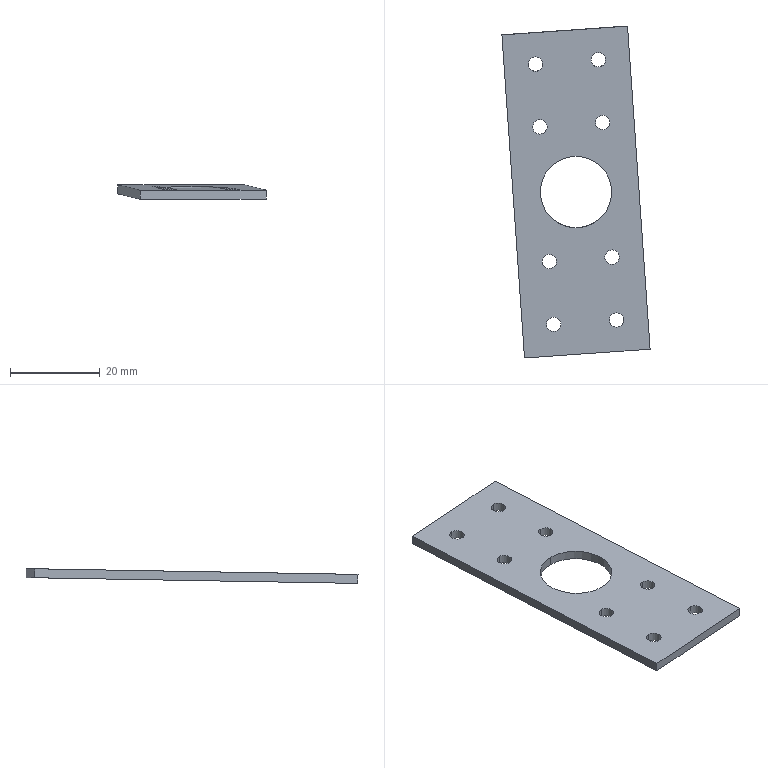Part | SolidWorks | features BaseBody 1 | 1 solid | 24 faces | box 32.959 x 73.801 x 3.287 mm | volume 3506 mm3 | cylinder 18 | plane 6 | commonest cylinder face diameters 3.2 x16 15.9 x2
STEP:
#1=CARTESIAN_POINT('',(561.633,59.844,3.845));
#2=VERTEX_POINT('',#1);
#3=CARTESIAN_POINT('',(561.633,43.947,3.568));
#4=VERTEX_POINT('',#3);
#5=CARTESIAN_POINT('',(561.633,51.896,3.706));
#6=DIRECTION('',(0.,-0.01745,0.9998));
#7=DIRECTION('',(0.,0.9998,0.01745));
#8=AXIS2_PLACEMENT_3D('',#5,#6,#7);
#9=CIRCLE('',#8,7.95);
#10=EDGE_CURVE('',#2,#4,#9,.T.);
#11=ORIENTED_EDGE('',*,*,#10,.T.);
#12=CARTESIAN_POINT('',(561.633,43.982,1.568));
#13=VERTEX_POINT('',#12);
#14=CARTESIAN_POINT('',(561.633,43.947,3.568));
#15=DIRECTION('',(0.,0.01745,-0.9998));
#16=VECTOR('',#15,1000.);
#17=LINE('',#14,#16);
#18=EDGE_CURVE('',#4,#13,#17,.T.);
#19=ORIENTED_EDGE('',*,*,#18,.T.);
#20=CARTESIAN_POINT('',(561.633,59.879,1.845));
#21=VERTEX_POINT('',#20);
#22=CARTESIAN_POINT('',(561.633,51.931,1.707));
#23=DIRECTION('',(0.,0.01745,-0.9998));
#24=DIRECTION('',(0.,0.9998,0.01745));
#25=AXIS2_PLACEMENT_3D('',#22,#23,#24);
#26=CIRCLE('',#25,7.95);
#27=EDGE_CURVE('',#13,#21,#26,.T.);
#28=ORIENTED_EDGE('',*,*,#27,.T.);
#29=CARTESIAN_POINT('',(561.633,59.844,3.845));
#30=DIRECTION('',(0.,0.01745,-0.9998));
#31=VECTOR('',#30,1000.);
#32=LINE('',#29,#31);
#33=EDGE_CURVE('',#2,#21,#32,.T.);
#34=ORIENTED_EDGE('',*,*,#33,.F.);
#35=EDGE_LOOP('',(#11,#19,#28,#34));
#36=FACE_OUTER_BOUND('',#35,.T.);
#37=CARTESIAN_POINT('',(561.633,51.896,3.706));
#38=DIRECTION('',(0.,0.01745,-0.9998));
#39=DIRECTION('',(0.,0.9998,0.01745));
#40=AXIS2_PLACEMENT_3D('',#37,#38,#39);
#41=CYLINDRICAL_SURFACE('',#40,7.95);
#42=ADVANCED_FACE('',(#36),#41,.F.);
#43=CARTESIAN_POINT('',(556.675,24.084,3.221));
#44=VERTEX_POINT('',#43);
#45=CARTESIAN_POINT('',(556.675,20.885,3.165));
#46=VERTEX_POINT('',#45);
#47=CARTESIAN_POINT('',(556.675,22.484,3.193));
#48=DIRECTION('',(0.,-0.01745,0.9998));
#49=DIRECTION('',(0.,0.9998,0.01745));
#50=AXIS2_PLACEMENT_3D('',#47,#48,#49);
#51=CIRCLE('',#50,1.6);
#52=EDGE_CURVE('',#44,#46,#51,.T.);
#53=ORIENTED_EDGE('',*,*,#52,.T.);
#54=CARTESIAN_POINT('',(556.675,20.92,1.165));
#55=VERTEX_POINT('',#54);
#56=CARTESIAN_POINT('',(556.675,20.885,3.165));
#57=DIRECTION('',(0.,0.01745,-0.9998));
#58=VECTOR('',#57,1000.);
#59=LINE('',#56,#58);
#60=EDGE_CURVE('',#46,#55,#59,.T.);
#61=ORIENTED_EDGE('',*,*,#60,.T.);
#62=CARTESIAN_POINT('',(556.675,24.119,1.221));
#63=VERTEX_POINT('',#62);
#64=CARTESIAN_POINT('',(556.675,22.519,1.193));
#65=DIRECTION('',(0.,-0.01745,0.9998));
#66=DIRECTION('',(0.,0.9998,0.01745));
#67=AXIS2_PLACEMENT_3D('',#64,#65,#66);
#68=CIRCLE('',#67,1.6);
#69=EDGE_CURVE('',#63,#55,#68,.T.);
#70=ORIENTED_EDGE('',*,*,#69,.F.);
#71=CARTESIAN_POINT('',(556.675,24.084,3.221));
#72=DIRECTION('',(0.,0.01745,-0.9998));
#73=VECTOR('',#72,1000.);
#74=LINE('',#71,#73);
#75=EDGE_CURVE('',#44,#63,#74,.T.);
#76=ORIENTED_EDGE('',*,*,#75,.F.);
#77=EDGE_LOOP('',(#53,#61,#70,#76));
#78=FACE_OUTER_BOUND('',#77,.T.);
#79=CARTESIAN_POINT('',(556.675,22.484,3.193));
#80=DIRECTION('',(0.,0.01745,-0.9998));
#81=DIRECTION('',(0.,0.9998,0.01745));
#82=AXIS2_PLACEMENT_3D('',#79,#80,#81);
#83=CYLINDRICAL_SURFACE('',#82,1.6);
#84=ADVANCED_FACE('',(#78),#83,.F.);
#85=CARTESIAN_POINT('',(555.698,38.048,3.465));
#86=VERTEX_POINT('',#85);
#87=CARTESIAN_POINT('',(555.698,34.848,3.409));
#88=VERTEX_POINT('',#87);
#89=CARTESIAN_POINT('',(555.698,36.448,3.437));
#90=DIRECTION('',(0.,-0.01745,0.9998));
#91=DIRECTION('',(0.,0.9998,0.01745));
#92=AXIS2_PLACEMENT_3D('',#89,#90,#91);
#93=CIRCLE('',#92,1.6);
#94=EDGE_CURVE('',#86,#88,#93,.T.);
#95=ORIENTED_EDGE('',*,*,#94,.T.);
#96=CARTESIAN_POINT('',(555.698,34.883,1.409));
#97=VERTEX_POINT('',#96);
#98=CARTESIAN_POINT('',(555.698,34.848,3.409));
#99=DIRECTION('',(0.,0.01745,-0.9998));
#100=VECTOR('',#99,1000.);
#101=LINE('',#98,#100);
#102=EDGE_CURVE('',#88,#97,#101,.T.);
#103=ORIENTED_EDGE('',*,*,#102,.T.);
#104=CARTESIAN_POINT('',(555.698,38.083,1.465));
#105=VERTEX_POINT('',#104);
#106=CARTESIAN_POINT('',(555.698,36.483,1.437));
#107=DIRECTION('',(0.,-0.01745,0.9998));
#108=DIRECTION('',(0.,0.9998,0.01745));
#109=AXIS2_PLACEMENT_3D('',#106,#107,#108);
#110=CIRCLE('',#109,1.6);
#111=EDGE_CURVE('',#105,#97,#110,.T.);
#112=ORIENTED_EDGE('',*,*,#111,.F.);
#113=CARTESIAN_POINT('',(555.698,38.048,3.465));
#114=DIRECTION('',(0.,0.01745,-0.9998));
#115=VECTOR('',#114,1000.);
#116=LINE('',#113,#115);
#117=EDGE_CURVE('',#86,#105,#116,.T.);
#118=ORIENTED_EDGE('',*,*,#117,.F.);
#119=EDGE_LOOP('',(#95,#103,#112,#118));
#120=FACE_OUTER_BOUND('',#119,.T.);
#121=CARTESIAN_POINT('',(555.698,36.448,3.437));
#122=DIRECTION('',(0.,0.01745,-0.9998));
#123=DIRECTION('',(0.,0.9998,0.01745));
#124=AXIS2_PLACEMENT_3D('',#121,#122,#123);
#125=CYLINDRICAL_SURFACE('',#124,1.6);
#126=ADVANCED_FACE('',(#120),#125,.F.);
#127=CARTESIAN_POINT('',(567.572,68.942,4.004));
#128=VERTEX_POINT('',#127);
#129=CARTESIAN_POINT('',(567.572,65.742,3.948));
#130=VERTEX_POINT('',#129);
#131=CARTESIAN_POINT('',(567.572,67.342,3.976));
#132=DIRECTION('',(0.,-0.01745,0.9998));
#133=DIRECTION('',(0.,0.9998,0.01745));
#134=AXIS2_PLACEMENT_3D('',#131,#132,#133);
#135=CIRCLE('',#134,1.6);
#136=EDGE_CURVE('',#128,#130,#135,.T.);
#137=ORIENTED_EDGE('',*,*,#136,.T.);
#138=CARTESIAN_POINT('',(567.572,65.777,1.948));
#139=VERTEX_POINT('',#138);
#140=CARTESIAN_POINT('',(567.572,65.742,3.948));
#141=DIRECTION('',(0.,0.01745,-0.9998));
#142=VECTOR('',#141,1000.);
#143=LINE('',#140,#142);
#144=EDGE_CURVE('',#130,#139,#143,.T.);
#145=ORIENTED_EDGE('',*,*,#144,.T.);
#146=CARTESIAN_POINT('',(567.572,68.977,2.004));
#147=VERTEX_POINT('',#146);
#148=CARTESIAN_POINT('',(567.572,67.377,1.976));
#149=DIRECTION('',(0.,-0.01745,0.9998));
#150=DIRECTION('',(0.,0.9998,0.01745));
#151=AXIS2_PLACEMENT_3D('',#148,#149,#150);
#152=CIRCLE('',#151,1.6);
#153=EDGE_CURVE('',#147,#139,#152,.T.);
#154=ORIENTED_EDGE('',*,*,#153,.F.);
#155=CARTESIAN_POINT('',(567.572,68.942,4.004));
#156=DIRECTION('',(0.,0.01745,-0.9998));
#157=VECTOR('',#156,1000.);
#158=LINE('',#155,#157);
#159=EDGE_CURVE('',#128,#147,#158,.T.);
#160=ORIENTED_EDGE('',*,*,#159,.F.);
#161=EDGE_LOOP('',(#137,#145,#154,#160));
#162=FACE_OUTER_BOUND('',#161,.T.);
#163=CARTESIAN_POINT('',(567.572,67.342,3.976));
#164=DIRECTION('',(0.,0.01745,-0.9998));
#165=DIRECTION('',(0.,0.9998,0.01745));
#166=AXIS2_PLACEMENT_3D('',#163,#164,#165);
#167=CYLINDRICAL_SURFACE('',#166,1.6);
#168=ADVANCED_FACE('',(#162),#167,.F.);
#169=CARTESIAN_POINT('',(566.596,82.906,4.248));
#170=VERTEX_POINT('',#169);
#171=CARTESIAN_POINT('',(566.596,79.706,4.192));
#172=VERTEX_POINT('',#171);
#173=CARTESIAN_POINT('',(566.596,81.306,4.22));
#174=DIRECTION('',(0.,-0.01745,0.9998));
#175=DIRECTION('',(0.,0.9998,0.01745));
#176=AXIS2_PLACEMENT_3D('',#173,#174,#175);
#177=CIRCLE('',#176,1.6);
#178=EDGE_CURVE('',#170,#172,#177,.T.);
#179=ORIENTED_EDGE('',*,*,#178,.T.);
#180=CARTESIAN_POINT('',(566.596,79.741,2.192));
#181=VERTEX_POINT('',#180);
#182=CARTESIAN_POINT('',(566.596,79.706,4.192));
#183=DIRECTION('',(0.,0.01745,-0.9998));
#184=VECTOR('',#183,1000.);
#185=LINE('',#182,#184);
#186=EDGE_CURVE('',#172,#181,#185,.T.);
#187=ORIENTED_EDGE('',*,*,#186,.T.);
#188=CARTESIAN_POINT('',(566.596,82.941,2.248));
#189=VERTEX_POINT('',#188);
#190=CARTESIAN_POINT('',(566.596,81.341,2.22));
#191=DIRECTION('',(0.,-0.01745,0.9998));
#192=DIRECTION('',(0.,0.9998,0.01745));
#193=AXIS2_PLACEMENT_3D('',#190,#191,#192);
#194=CIRCLE('',#193,1.6);
#195=EDGE_CURVE('',#189,#181,#194,.T.);
#196=ORIENTED_EDGE('',*,*,#195,.F.);
#197=CARTESIAN_POINT('',(566.596,82.906,4.248));
#198=DIRECTION('',(0.,0.01745,-0.9998));
#199=VECTOR('',#198,1000.);
#200=LINE('',#197,#199);
#201=EDGE_CURVE('',#170,#189,#200,.T.);
#202=ORIENTED_EDGE('',*,*,#201,.F.);
#203=EDGE_LOOP('',(#179,#187,#196,#202));
#204=FACE_OUTER_BOUND('',#203,.T.);
#205=CARTESIAN_POINT('',(566.596,81.306,4.22));
#206=DIRECTION('',(0.,0.01745,-0.9998));
#207=DIRECTION('',(0.,0.9998,0.01745));
#208=AXIS2_PLACEMENT_3D('',#205,#206,#207);
#209=CYLINDRICAL_SURFACE('',#208,1.6);
#210=ADVANCED_FACE('',(#204),#209,.F.);
#211=CARTESIAN_POINT('',(552.63,81.931,4.231));
#212=VERTEX_POINT('',#211);
#213=CARTESIAN_POINT('',(552.63,78.731,4.175));
#214=VERTEX_POINT('',#213);
#215=CARTESIAN_POINT('',(552.63,80.331,4.203));
#216=DIRECTION('',(0.,-0.01745,0.9998));
#217=DIRECTION('',(0.,0.9998,0.01745));
#218=AXIS2_PLACEMENT_3D('',#215,#216,#217);
#219=CIRCLE('',#218,1.6);
#220=EDGE_CURVE('',#212,#214,#219,.T.);
#221=ORIENTED_EDGE('',*,*,#220,.T.);
#222=CARTESIAN_POINT('',(552.63,78.766,2.175));
#223=VERTEX_POINT('',#222);
#224=CARTESIAN_POINT('',(552.63,78.731,4.175));
#225=DIRECTION('',(0.,0.01745,-0.9998));
#226=VECTOR('',#225,1000.);
#227=LINE('',#224,#226);
#228=EDGE_CURVE('',#214,#223,#227,.T.);
#229=ORIENTED_EDGE('',*,*,#228,.T.);
#230=CARTESIAN_POINT('',(552.63,81.966,2.231));
#231=VERTEX_POINT('',#230);
#232=CARTESIAN_POINT('',(552.63,80.366,2.203));
#233=DIRECTION('',(0.,-0.01745,0.9998));
#234=DIRECTION('',(0.,0.9998,0.01745));
#235=AXIS2_PLACEMENT_3D('',#232,#233,#234);
#236=CIRCLE('',#235,1.6);
#237=EDGE_CURVE('',#231,#223,#236,.T.);
#238=ORIENTED_EDGE('',*,*,#237,.F.);
#239=CARTESIAN_POINT('',(552.63,81.931,4.231));
#240=DIRECTION('',(0.,0.01745,-0.9998));
#241=VECTOR('',#240,1000.);
#242=LINE('',#239,#241);
#243=EDGE_CURVE('',#212,#231,#242,.T.);
#244=ORIENTED_EDGE('',*,*,#243,.F.);
#245=EDGE_LOOP('',(#221,#229,#238,#244));
#246=FACE_OUTER_BOUND('',#245,.T.);
#247=CARTESIAN_POINT('',(552.63,80.331,4.203));
#248=DIRECTION('',(0.,0.01745,-0.9998));
#249=DIRECTION('',(0.,0.9998,0.01745));
#250=AXIS2_PLACEMENT_3D('',#247,#248,#249);
#251=CYLINDRICAL_SURFACE('',#250,1.6);
#252=ADVANCED_FACE('',(#246),#251,.F.);
#253=CARTESIAN_POINT('',(553.606,67.967,3.987));
#254=VERTEX_POINT('',#253);
#255=CARTESIAN_POINT('',(553.606,64.767,3.931));
#256=VERTEX_POINT('',#255);
#257=CARTESIAN_POINT('',(553.606,66.367,3.959));
#258=DIRECTION('',(0.,-0.01745,0.9998));
#259=DIRECTION('',(0.,0.9998,0.01745));
#260=AXIS2_PLACEMENT_3D('',#257,#258,#259);
#261=CIRCLE('',#260,1.6);
#262=EDGE_CURVE('',#254,#256,#261,.T.);
#263=ORIENTED_EDGE('',*,*,#262,.T.);
#264=CARTESIAN_POINT('',(553.606,64.802,1.931));
#265=VERTEX_POINT('',#264);
#266=CARTESIAN_POINT('',(553.606,64.767,3.931));
#267=DIRECTION('',(0.,0.01745,-0.9998));
#268=VECTOR('',#267,1000.);
#269=LINE('',#266,#268);
#270=EDGE_CURVE('',#256,#265,#269,.T.);
#271=ORIENTED_EDGE('',*,*,#270,.T.);
#272=CARTESIAN_POINT('',(553.606,68.002,1.987));
#273=VERTEX_POINT('',#272);
#274=CARTESIAN_POINT('',(553.606,66.402,1.959));
#275=DIRECTION('',(0.,-0.01745,0.9998));
#276=DIRECTION('',(0.,0.9998,0.01745));
#277=AXIS2_PLACEMENT_3D('',#274,#275,#276);
#278=CIRCLE('',#277,1.6);
#279=EDGE_CURVE('',#273,#265,#278,.T.);
#280=ORIENTED_EDGE('',*,*,#279,.F.);
#281=CARTESIAN_POINT('',(553.606,67.967,3.987));
#282=DIRECTION('',(0.,0.01745,-0.9998));
#283=VECTOR('',#282,1000.);
#284=LINE('',#281,#283);
#285=EDGE_CURVE('',#254,#273,#284,.T.);
#286=ORIENTED_EDGE('',*,*,#285,.F.);
#287=EDGE_LOOP('',(#263,#271,#280,#286));
#288=FACE_OUTER_BOUND('',#287,.T.);
#289=CARTESIAN_POINT('',(553.606,66.367,3.959));
#290=DIRECTION('',(0.,0.01745,-0.9998));
#291=DIRECTION('',(0.,0.9998,0.01745));
#292=AXIS2_PLACEMENT_3D('',#289,#290,#291);
#293=CYLINDRICAL_SURFACE('',#292,1.6);
#294=ADVANCED_FACE('',(#288),#293,.F.);
#295=CARTESIAN_POINT('',(569.663,39.025,3.482));
#296=VERTEX_POINT('',#295);
#297=CARTESIAN_POINT('',(569.663,35.826,3.426));
#298=VERTEX_POINT('',#297);
#299=CARTESIAN_POINT('',(569.663,37.425,3.454));
#300=DIRECTION('',(0.,-0.01745,0.9998));
#301=DIRECTION('',(0.,0.9998,0.01745));
#302=AXIS2_PLACEMENT_3D('',#299,#300,#301);
#303=CIRCLE('',#302,1.6);
#304=EDGE_CURVE('',#296,#298,#303,.T.);
#305=ORIENTED_EDGE('',*,*,#304,.T.);
#306=CARTESIAN_POINT('',(569.663,35.861,1.426));
#307=VERTEX_POINT('',#306);
#308=CARTESIAN_POINT('',(569.663,35.826,3.426));
#309=DIRECTION('',(0.,0.01745,-0.9998));
#310=VECTOR('',#309,1000.);
#311=LINE('',#308,#310);
#312=EDGE_CURVE('',#298,#307,#311,.T.);
#313=ORIENTED_EDGE('',*,*,#312,.T.);
#314=CARTESIAN_POINT('',(569.663,39.06,1.482));
#315=VERTEX_POINT('',#314);
#316=CARTESIAN_POINT('',(569.663,37.46,1.454));
#317=DIRECTION('',(0.,-0.01745,0.9998));
#318=DIRECTION('',(0.,0.9998,0.01745));
#319=AXIS2_PLACEMENT_3D('',#316,#317,#318);
#320=CIRCLE('',#319,1.6);
#321=EDGE_CURVE('',#315,#307,#320,.T.);
#322=ORIENTED_EDGE('',*,*,#321,.F.);
#323=CARTESIAN_POINT('',(569.663,39.025,3.482));
#324=DIRECTION('',(0.,0.01745,-0.9998));
#325=VECTOR('',#324,1000.);
#326=LINE('',#323,#325);
#327=EDGE_CURVE('',#296,#315,#326,.T.);
#328=ORIENTED_EDGE('',*,*,#327,.F.);
#329=EDGE_LOOP('',(#305,#313,#322,#328));
#330=FACE_OUTER_BOUND('',#329,.T.);
#331=CARTESIAN_POINT('',(569.663,37.425,3.454));
#332=DIRECTION('',(0.,0.01745,-0.9998));
#333=DIRECTION('',(0.,0.9998,0.01745));
#334=AXIS2_PLACEMENT_3D('',#331,#332,#333);
#335=CYLINDRICAL_SURFACE('',#334,1.6);
#336=ADVANCED_FACE('',(#330),#335,.F.);
#337=CARTESIAN_POINT('',(570.641,25.062,3.238));
#338=VERTEX_POINT('',#337);
#339=CARTESIAN_POINT('',(570.641,21.862,3.182));
#340=VERTEX_POINT('',#339);
#341=CARTESIAN_POINT('',(570.641,23.462,3.21));
#342=DIRECTION('',(0.,-0.01745,0.9998));
#343=DIRECTION('',(0.,0.9998,0.01745));
#344=AXIS2_PLACEMENT_3D('',#341,#342,#343);
#345=CIRCLE('',#344,1.6);
#346=EDGE_CURVE('',#338,#340,#345,.T.);
#347=ORIENTED_EDGE('',*,*,#346,.T.);
#348=CARTESIAN_POINT('',(570.641,21.897,1.182));
#349=VERTEX_POINT('',#348);
#350=CARTESIAN_POINT('',(570.641,21.862,3.182));
#351=DIRECTION('',(0.,0.01745,-0.9998));
#352=VECTOR('',#351,1000.);
#353=LINE('',#350,#352);
#354=EDGE_CURVE('',#340,#349,#353,.T.);
#355=ORIENTED_EDGE('',*,*,#354,.T.);
#356=CARTESIAN_POINT('',(570.641,25.096,1.238));
#357=VERTEX_POINT('',#356);
#358=CARTESIAN_POINT('',(570.641,23.497,1.21));
#359=DIRECTION('',(0.,-0.01745,0.9998));
#360=DIRECTION('',(0.,0.9998,0.01745));
#361=AXIS2_PLACEMENT_3D('',#358,#359,#360);
#362=CIRCLE('',#361,1.6);
#363=EDGE_CURVE('',#357,#349,#362,.T.);
#364=ORIENTED_EDGE('',*,*,#363,.F.);
#365=CARTESIAN_POINT('',(570.641,25.062,3.238));
#366=DIRECTION('',(0.,0.01745,-0.9998));
#367=VECTOR('',#366,1000.);
#368=LINE('',#365,#367);
#369=EDGE_CURVE('',#338,#357,#368,.T.);
#370=ORIENTED_EDGE('',*,*,#369,.F.);
#371=EDGE_LOOP('',(#347,#355,#364,#370));
#372=FACE_OUTER_BOUND('',#371,.T.);
#373=CARTESIAN_POINT('',(570.641,23.462,3.21));
#374=DIRECTION('',(0.,0.01745,-0.9998));
#375=DIRECTION('',(0.,0.9998,0.01745));
#376=AXIS2_PLACEMENT_3D('',#373,#374,#375);
#377=CYLINDRICAL_SURFACE('',#376,1.6);
#378=ADVANCED_FACE('',(#372),#377,.F.);
#379=ORIENTED_EDGE('',*,*,#18,.F.);
#380=CARTESIAN_POINT('',(561.633,51.896,3.706));
#381=DIRECTION('',(0.,-0.01745,0.9998));
#382=DIRECTION('',(0.,0.9998,0.01745));
#383=AXIS2_PLACEMENT_3D('',#380,#381,#382);
#384=CIRCLE('',#383,7.95);
#385=EDGE_CURVE('',#4,#2,#384,.T.);
#386=ORIENTED_EDGE('',*,*,#385,.T.);
#387=ORIENTED_EDGE('',*,*,#33,.T.);
#388=CARTESIAN_POINT('',(561.633,51.931,1.707));
#389=DIRECTION('',(0.,0.01745,-0.9998));
#390=DIRECTION('',(0.,0.9998,0.01745));
#391=AXIS2_PLACEMENT_3D('',#388,#389,#390);
#392=CIRCLE('',#391,7.95);
#393=EDGE_CURVE('',#21,#13,#392,.T.);
#394=ORIENTED_EDGE('',*,*,#393,.T.);
#395=EDGE_LOOP('',(#379,#386,#387,#394));
#396=FACE_OUTER_BOUND('',#395,.T.);
#397=CARTESIAN_POINT('',(561.633,51.896,3.706));
#398=DIRECTION('',(0.,0.01745,-0.9998));
#399=DIRECTION('',(0.,0.9998,0.01745));
#400=AXIS2_PLACEMENT_3D('',#397,#398,#399);
#401=CYLINDRICAL_SURFACE('',#400,7.95);
#402=ADVANCED_FACE('',(#396),#401,.F.);
#403=ORIENTED_EDGE('',*,*,#393,.F.);
#404=ORIENTED_EDGE('',*,*,#27,.F.);
#405=EDGE_LOOP('',(#403,#404));
#406=FACE_BOUND('',#405,.T.);
#407=ORIENTED_EDGE('',*,*,#69,.T.);
#408=CARTESIAN_POINT('',(556.675,22.519,1.193));
#409=DIRECTION('',(0.,-0.01745,0.9998));
#410=DIRECTION('',(0.,0.9998,0.01745));
#411=AXIS2_PLACEMENT_3D('',#408,#409,#410);
#412=CIRCLE('',#411,1.6);
#413=EDGE_CURVE('',#55,#63,#412,.T.);
#414=ORIENTED_EDGE('',*,*,#413,.T.);
#415=EDGE_LOOP('',(#407,#414));
#416=FACE_BOUND('',#415,.T.);
#417=ORIENTED_EDGE('',*,*,#111,.T.);
#418=CARTESIAN_POINT('',(555.698,36.483,1.437));
#419=DIRECTION('',(0.,-0.01745,0.9998));
#420=DIRECTION('',(0.,0.9998,0.01745));
#421=AXIS2_PLACEMENT_3D('',#418,#419,#420);
#422=CIRCLE('',#421,1.6);
#423=EDGE_CURVE('',#97,#105,#422,.T.);
#424=ORIENTED_EDGE('',*,*,#423,.T.);
#425=EDGE_LOOP('',(#417,#424));
#426=FACE_BOUND('',#425,.T.);
#427=ORIENTED_EDGE('',*,*,#153,.T.);
#428=CARTESIAN_POINT('',(567.572,67.377,1.976));
#429=DIRECTION('',(0.,-0.01745,0.9998));
#430=DIRECTION('',(0.,0.9998,0.01745));
#431=AXIS2_PLACEMENT_3D('',#428,#429,#430);
#432=CIRCLE('',#431,1.6);
#433=EDGE_CURVE('',#139,#147,#432,.T.);
#434=ORIENTED_EDGE('',*,*,#433,.T.);
#435=EDGE_LOOP('',(#427,#434));
#436=FACE_BOUND('',#435,.T.);
#437=ORIENTED_EDGE('',*,*,#195,.T.);
#438=CARTESIAN_POINT('',(566.596,81.341,2.22));
#439=DIRECTION('',(0.,-0.01745,0.9998));
#440=DIRECTION('',(0.,0.9998,0.01745));
#441=AXIS2_PLACEMENT_3D('',#438,#439,#440);
#442=CIRCLE('',#441,1.6);
#443=EDGE_CURVE('',#181,#189,#442,.T.);
#444=ORIENTED_EDGE('',*,*,#443,.T.);
#445=EDGE_LOOP('',(#437,#444));
#446=FACE_BOUND('',#445,.T.);
#447=ORIENTED_EDGE('',*,*,#237,.T.);
#448=CARTESIAN_POINT('',(552.63,80.366,2.203));
#449=DIRECTION('',(0.,-0.01745,0.9998));
#450=DIRECTION('',(0.,0.9998,0.01745));
#451=AXIS2_PLACEMENT_3D('',#448,#449,#450);
#452=CIRCLE('',#451,1.6);
#453=EDGE_CURVE('',#223,#231,#452,.T.);
#454=ORIENTED_EDGE('',*,*,#453,.T.);
#455=EDGE_LOOP('',(#447,#454));
#456=FACE_BOUND('',#455,.T.);
#457=ORIENTED_EDGE('',*,*,#279,.T.);
#458=CARTESIAN_POINT('',(553.606,66.402,1.959));
#459=DIRECTION('',(0.,-0.01745,0.9998));
#460=DIRECTION('',(0.,0.9998,0.01745));
#461=AXIS2_PLACEMENT_3D('',#458,#459,#460);
#462=CIRCLE('',#461,1.6);
#463=EDGE_CURVE('',#265,#273,#462,.T.);
#464=ORIENTED_EDGE('',*,*,#463,.T.);
#465=EDGE_LOOP('',(#457,#464));
#466=FACE_BOUND('',#465,.T.);
#467=ORIENTED_EDGE('',*,*,#321,.T.);
#468=CARTESIAN_POINT('',(569.663,37.46,1.454));
#469=DIRECTION('',(0.,-0.01745,0.9998));
#470=DIRECTION('',(0.,0.9998,0.01745));
#471=AXIS2_PLACEMENT_3D('',#468,#469,#470);
#472=CIRCLE('',#471,1.6);
#473=EDGE_CURVE('',#307,#315,#472,.T.);
#474=ORIENTED_EDGE('',*,*,#473,.T.);
#475=EDGE_LOOP('',(#467,#474));
#476=FACE_BOUND('',#475,.T.);
#477=ORIENTED_EDGE('',*,*,#363,.T.);
#478=CARTESIAN_POINT('',(570.641,23.497,1.21));
#479=DIRECTION('',(0.,-0.01745,0.9998));
#480=DIRECTION('',(0.,0.9998,0.01745));
#481=AXIS2_PLACEMENT_3D('',#478,#479,#480);
#482=CIRCLE('',#481,1.6);
#483=EDGE_CURVE('',#349,#357,#482,.T.);
#484=ORIENTED_EDGE('',*,*,#483,.T.);
#485=EDGE_LOOP('',(#477,#484));
#486=FACE_BOUND('',#485,.T.);
#487=CARTESIAN_POINT('',(550.181,15.049,1.063));
#488=VERTEX_POINT('',#487);
#489=CARTESIAN_POINT('',(545.154,86.86,2.316));
#490=VERTEX_POINT('',#489);
#491=CARTESIAN_POINT('',(550.181,15.049,1.063));
#492=DIRECTION('',(-0.06982,0.9974,0.01741));
#493=VECTOR('',#492,1000.);
#494=LINE('',#491,#493);
#495=EDGE_CURVE('',#488,#490,#494,.T.);
#496=ORIENTED_EDGE('',*,*,#495,.T.);
#497=CARTESIAN_POINT('',(573.086,88.815,2.35));
#498=VERTEX_POINT('',#497);
#499=CARTESIAN_POINT('',(545.154,86.86,2.316));
#500=DIRECTION('',(0.9976,0.06981,0.001219));
#501=VECTOR('',#500,1000.);
#502=LINE('',#499,#501);
#503=EDGE_CURVE('',#490,#498,#502,.T.);
#504=ORIENTED_EDGE('',*,*,#503,.T.);
#505=CARTESIAN_POINT('',(578.113,17.003,1.097));
#506=VERTEX_POINT('',#505);
#507=CARTESIAN_POINT('',(573.086,88.815,2.35));
#508=DIRECTION('',(0.06982,-0.9974,-0.01741));
#509=VECTOR('',#508,1000.);
#510=LINE('',#507,#509);
#511=EDGE_CURVE('',#498,#506,#510,.T.);
#512=ORIENTED_EDGE('',*,*,#511,.T.);
#513=CARTESIAN_POINT('',(578.113,17.003,1.097));
#514=DIRECTION('',(-0.9976,-0.06981,-0.001219));
#515=VECTOR('',#514,1000.);
#516=LINE('',#513,#515);
#517=EDGE_CURVE('',#506,#488,#516,.T.);
#518=ORIENTED_EDGE('',*,*,#517,.T.);
#519=EDGE_LOOP('',(#496,#504,#512,#518));
#520=FACE_OUTER_BOUND('',#519,.T.);
#521=CARTESIAN_POINT('',(544.956,14.606,1.055));
#522=DIRECTION('',(0.,0.01745,-0.9998));
#523=DIRECTION('',(0.,0.9998,0.01745));
#524=AXIS2_PLACEMENT_3D('',#521,#522,#523);
#525=PLANE('',#524);
#526=ADVANCED_FACE('',(#406,#416,#426,#436,#446,#456,#466,#476,#486,#520),#525,.T.);
#527=ORIENTED_EDGE('',*,*,#10,.F.);
#528=ORIENTED_EDGE('',*,*,#385,.F.);
#529=EDGE_LOOP('',(#527,#528));
#530=FACE_BOUND('',#529,.T.);
#531=ORIENTED_EDGE('',*,*,#52,.F.);
#532=CARTESIAN_POINT('',(556.675,22.484,3.193));
#533=DIRECTION('',(0.,-0.01745,0.9998));
#534=DIRECTION('',(0.,0.9998,0.01745));
#535=AXIS2_PLACEMENT_3D('',#532,#533,#534);
#536=CIRCLE('',#535,1.6);
#537=EDGE_CURVE('',#46,#44,#536,.T.);
#538=ORIENTED_EDGE('',*,*,#537,.F.);
#539=EDGE_LOOP('',(#531,#538));
#540=FACE_BOUND('',#539,.T.);
#541=ORIENTED_EDGE('',*,*,#94,.F.);
#542=CARTESIAN_POINT('',(555.698,36.448,3.437));
#543=DIRECTION('',(0.,-0.01745,0.9998));
#544=DIRECTION('',(0.,0.9998,0.01745));
#545=AXIS2_PLACEMENT_3D('',#542,#543,#544);
#546=CIRCLE('',#545,1.6);
#547=EDGE_CURVE('',#88,#86,#546,.T.);
#548=ORIENTED_EDGE('',*,*,#547,.F.);
#549=EDGE_LOOP('',(#541,#548));
#550=FACE_BOUND('',#549,.T.);
#551=ORIENTED_EDGE('',*,*,#136,.F.);
#552=CARTESIAN_POINT('',(567.572,67.342,3.976));
#553=DIRECTION('',(0.,-0.01745,0.9998));
#554=DIRECTION('',(0.,0.9998,0.01745));
#555=AXIS2_PLACEMENT_3D('',#552,#553,#554);
#556=CIRCLE('',#555,1.6);
#557=EDGE_CURVE('',#130,#128,#556,.T.);
#558=ORIENTED_EDGE('',*,*,#557,.F.);
#559=EDGE_LOOP('',(#551,#558));
#560=FACE_BOUND('',#559,.T.);
#561=ORIENTED_EDGE('',*,*,#178,.F.);
#562=CARTESIAN_POINT('',(566.596,81.306,4.22));
#563=DIRECTION('',(0.,-0.01745,0.9998));
#564=DIRECTION('',(0.,0.9998,0.01745));
#565=AXIS2_PLACEMENT_3D('',#562,#563,#564);
#566=CIRCLE('',#565,1.6);
#567=EDGE_CURVE('',#172,#170,#566,.T.);
#568=ORIENTED_EDGE('',*,*,#567,.F.);
#569=EDGE_LOOP('',(#561,#568));
#570=FACE_BOUND('',#569,.T.);
#571=ORIENTED_EDGE('',*,*,#220,.F.);
#572=CARTESIAN_POINT('',(552.63,80.331,4.203));
#573=DIRECTION('',(0.,-0.01745,0.9998));
#574=DIRECTION('',(0.,0.9998,0.01745));
#575=AXIS2_PLACEMENT_3D('',#572,#573,#574);
#576=CIRCLE('',#575,1.6);
#577=EDGE_CURVE('',#214,#212,#576,.T.);
#578=ORIENTED_EDGE('',*,*,#577,.F.);
#579=EDGE_LOOP('',(#571,#578));
#580=FACE_BOUND('',#579,.T.);
#581=ORIENTED_EDGE('',*,*,#262,.F.);
#582=CARTESIAN_POINT('',(553.606,66.367,3.959));
#583=DIRECTION('',(0.,-0.01745,0.9998));
#584=DIRECTION('',(0.,0.9998,0.01745));
#585=AXIS2_PLACEMENT_3D('',#582,#583,#584);
#586=CIRCLE('',#585,1.6);
#587=EDGE_CURVE('',#256,#254,#586,.T.);
#588=ORIENTED_EDGE('',*,*,#587,.F.);
#589=EDGE_LOOP('',(#581,#588));
#590=FACE_BOUND('',#589,.T.);
#591=ORIENTED_EDGE('',*,*,#304,.F.);
#592=CARTESIAN_POINT('',(569.663,37.425,3.454));
#593=DIRECTION('',(0.,-0.01745,0.9998));
#594=DIRECTION('',(0.,0.9998,0.01745));
#595=AXIS2_PLACEMENT_3D('',#592,#593,#594);
#596=CIRCLE('',#595,1.6);
#597=EDGE_CURVE('',#298,#296,#596,.T.);
#598=ORIENTED_EDGE('',*,*,#597,.F.);
#599=EDGE_LOOP('',(#591,#598));
#600=FACE_BOUND('',#599,.T.);
#601=ORIENTED_EDGE('',*,*,#346,.F.);
#602=CARTESIAN_POINT('',(570.641,23.462,3.21));
#603=DIRECTION('',(0.,-0.01745,0.9998));
#604=DIRECTION('',(0.,0.9998,0.01745));
#605=AXIS2_PLACEMENT_3D('',#602,#603,#604);
#606=CIRCLE('',#605,1.6);
#607=EDGE_CURVE('',#340,#338,#606,.T.);
#608=ORIENTED_EDGE('',*,*,#607,.F.);
#609=EDGE_LOOP('',(#601,#608));
#610=FACE_BOUND('',#609,.T.);
#611=CARTESIAN_POINT('',(545.154,86.825,4.316));
#612=VERTEX_POINT('',#611);
#613=CARTESIAN_POINT('',(573.086,88.78,4.35));
#614=VERTEX_POINT('',#613);
#615=CARTESIAN_POINT('',(545.154,86.825,4.316));
#616=DIRECTION('',(0.9976,0.06981,0.001219));
#617=VECTOR('',#616,1000.);
#618=LINE('',#615,#617);
#619=EDGE_CURVE('',#612,#614,#618,.T.);
#620=ORIENTED_EDGE('',*,*,#619,.F.);
#621=CARTESIAN_POINT('',(550.181,15.014,3.062));
#622=VERTEX_POINT('',#621);
#623=CARTESIAN_POINT('',(550.181,15.014,3.062));
#624=DIRECTION('',(-0.06982,0.9974,0.01741));
#625=VECTOR('',#624,1000.);
#626=LINE('',#623,#625);
#627=EDGE_CURVE('',#622,#612,#626,.T.);
#628=ORIENTED_EDGE('',*,*,#627,.F.);
#629=CARTESIAN_POINT('',(578.113,16.969,3.097));
#630=VERTEX_POINT('',#629);
#631=CARTESIAN_POINT('',(578.113,16.969,3.097));
#632=DIRECTION('',(-0.9976,-0.06981,-0.001219));
#633=VECTOR('',#632,1000.);
#634=LINE('',#631,#633);
#635=EDGE_CURVE('',#630,#622,#634,.T.);
#636=ORIENTED_EDGE('',*,*,#635,.F.);
#637=CARTESIAN_POINT('',(573.086,88.78,4.35));
#638=DIRECTION('',(0.06982,-0.9974,-0.01741));
#639=VECTOR('',#638,1000.);
#640=LINE('',#637,#639);
#641=EDGE_CURVE('',#614,#630,#640,.T.);
#642=ORIENTED_EDGE('',*,*,#641,.F.);
#643=EDGE_LOOP('',(#620,#628,#636,#642));
#644=FACE_OUTER_BOUND('',#643,.T.);
#645=CARTESIAN_POINT('',(544.956,14.571,3.055));
#646=DIRECTION('',(0.,0.01745,-0.9998));
#647=DIRECTION('',(0.,0.9998,0.01745));
#648=AXIS2_PLACEMENT_3D('',#645,#646,#647);
#649=PLANE('',#648);
#650=ADVANCED_FACE('',(#530,#540,#550,#560,#570,#580,#590,#600,#610,#644),#649,.F.);
#651=ORIENTED_EDGE('',*,*,#60,.F.);
#652=ORIENTED_EDGE('',*,*,#537,.T.);
#653=ORIENTED_EDGE('',*,*,#75,.T.);
#654=ORIENTED_EDGE('',*,*,#413,.F.);
#655=EDGE_LOOP('',(#651,#652,#653,#654));
#656=FACE_OUTER_BOUND('',#655,.T.);
#657=CARTESIAN_POINT('',(556.675,22.484,3.193));
#658=DIRECTION('',(0.,0.01745,-0.9998));
#659=DIRECTION('',(0.,0.9998,0.01745));
#660=AXIS2_PLACEMENT_3D('',#657,#658,#659);
#661=CYLINDRICAL_SURFACE('',#660,1.6);
#662=ADVANCED_FACE('',(#656),#661,.F.);
#663=ORIENTED_EDGE('',*,*,#102,.F.);
#664=ORIENTED_EDGE('',*,*,#547,.T.);
#665=ORIENTED_EDGE('',*,*,#117,.T.);
#666=ORIENTED_EDGE('',*,*,#423,.F.);
#667=EDGE_LOOP('',(#663,#664,#665,#666));
#668=FACE_OUTER_BOUND('',#667,.T.);
#669=CARTESIAN_POINT('',(555.698,36.448,3.437));
#670=DIRECTION('',(0.,0.01745,-0.9998));
#671=DIRECTION('',(0.,0.9998,0.01745));
#672=AXIS2_PLACEMENT_3D('',#669,#670,#671);
#673=CYLINDRICAL_SURFACE('',#672,1.6);
#674=ADVANCED_FACE('',(#668),#673,.F.);
#675=ORIENTED_EDGE('',*,*,#144,.F.);
#676=ORIENTED_EDGE('',*,*,#557,.T.);
#677=ORIENTED_EDGE('',*,*,#159,.T.);
#678=ORIENTED_EDGE('',*,*,#433,.F.);
#679=EDGE_LOOP('',(#675,#676,#677,#678));
#680=FACE_OUTER_BOUND('',#679,.T.);
#681=CARTESIAN_POINT('',(567.572,67.342,3.976));
#682=DIRECTION('',(0.,0.01745,-0.9998));
#683=DIRECTION('',(0.,0.9998,0.01745));
#684=AXIS2_PLACEMENT_3D('',#681,#682,#683);
#685=CYLINDRICAL_SURFACE('',#684,1.6);
#686=ADVANCED_FACE('',(#680),#685,.F.);
#687=ORIENTED_EDGE('',*,*,#186,.F.);
#688=ORIENTED_EDGE('',*,*,#567,.T.);
#689=ORIENTED_EDGE('',*,*,#201,.T.);
#690=ORIENTED_EDGE('',*,*,#443,.F.);
#691=EDGE_LOOP('',(#687,#688,#689,#690));
#692=FACE_OUTER_BOUND('',#691,.T.);
#693=CARTESIAN_POINT('',(566.596,81.306,4.22));
#694=DIRECTION('',(0.,0.01745,-0.9998));
#695=DIRECTION('',(0.,0.9998,0.01745));
#696=AXIS2_PLACEMENT_3D('',#693,#694,#695);
#697=CYLINDRICAL_SURFACE('',#696,1.6);
#698=ADVANCED_FACE('',(#692),#697,.F.);
#699=ORIENTED_EDGE('',*,*,#228,.F.);
#700=ORIENTED_EDGE('',*,*,#577,.T.);
#701=ORIENTED_EDGE('',*,*,#243,.T.);
#702=ORIENTED_EDGE('',*,*,#453,.F.);
#703=EDGE_LOOP('',(#699,#700,#701,#702));
#704=FACE_OUTER_BOUND('',#703,.T.);
#705=CARTESIAN_POINT('',(552.63,80.331,4.203));
#706=DIRECTION('',(0.,0.01745,-0.9998));
#707=DIRECTION('',(0.,0.9998,0.01745));
#708=AXIS2_PLACEMENT_3D('',#705,#706,#707);
#709=CYLINDRICAL_SURFACE('',#708,1.6);
#710=ADVANCED_FACE('',(#704),#709,.F.);
#711=ORIENTED_EDGE('',*,*,#270,.F.);
#712=ORIENTED_EDGE('',*,*,#587,.T.);
#713=ORIENTED_EDGE('',*,*,#285,.T.);
#714=ORIENTED_EDGE('',*,*,#463,.F.);
#715=EDGE_LOOP('',(#711,#712,#713,#714));
#716=FACE_OUTER_BOUND('',#715,.T.);
#717=CARTESIAN_POINT('',(553.606,66.367,3.959));
#718=DIRECTION('',(0.,0.01745,-0.9998));
#719=DIRECTION('',(0.,0.9998,0.01745));
#720=AXIS2_PLACEMENT_3D('',#717,#718,#719);
#721=CYLINDRICAL_SURFACE('',#720,1.6);
#722=ADVANCED_FACE('',(#716),#721,.F.);
#723=ORIENTED_EDGE('',*,*,#312,.F.);
#724=ORIENTED_EDGE('',*,*,#597,.T.);
#725=ORIENTED_EDGE('',*,*,#327,.T.);
#726=ORIENTED_EDGE('',*,*,#473,.F.);
#727=EDGE_LOOP('',(#723,#724,#725,#726));
#728=FACE_OUTER_BOUND('',#727,.T.);
#729=CARTESIAN_POINT('',(569.663,37.425,3.454));
#730=DIRECTION('',(0.,0.01745,-0.9998));
#731=DIRECTION('',(0.,0.9998,0.01745));
#732=AXIS2_PLACEMENT_3D('',#729,#730,#731);
#733=CYLINDRICAL_SURFACE('',#732,1.6);
#734=ADVANCED_FACE('',(#728),#733,.F.);
#735=ORIENTED_EDGE('',*,*,#354,.F.);
#736=ORIENTED_EDGE('',*,*,#607,.T.);
#737=ORIENTED_EDGE('',*,*,#369,.T.);
#738=ORIENTED_EDGE('',*,*,#483,.F.);
#739=EDGE_LOOP('',(#735,#736,#737,#738));
#740=FACE_OUTER_BOUND('',#739,.T.);
#741=CARTESIAN_POINT('',(570.641,23.462,3.21));
#742=DIRECTION('',(0.,0.01745,-0.9998));
#743=DIRECTION('',(0.,0.9998,0.01745));
#744=AXIS2_PLACEMENT_3D('',#741,#742,#743);
#745=CYLINDRICAL_SURFACE('',#744,1.6);
#746=ADVANCED_FACE('',(#740),#745,.F.);
#747=CARTESIAN_POINT('',(545.154,86.825,4.316));
#748=DIRECTION('',(0.,0.01745,-0.9998));
#749=VECTOR('',#748,1000.);
#750=LINE('',#747,#749);
#751=EDGE_CURVE('',#612,#490,#750,.T.);
#752=ORIENTED_EDGE('',*,*,#751,.F.);
#753=ORIENTED_EDGE('',*,*,#619,.T.);
#754=CARTESIAN_POINT('',(573.086,88.815,2.35));
#755=DIRECTION('',(0.,-0.01745,0.9998));
#756=VECTOR('',#755,1000.);
#757=LINE('',#754,#756);
#758=EDGE_CURVE('',#498,#614,#757,.T.);
#759=ORIENTED_EDGE('',*,*,#758,.F.);
#760=ORIENTED_EDGE('',*,*,#503,.F.);
#761=EDGE_LOOP('',(#752,#753,#759,#760));
#762=FACE_OUTER_BOUND('',#761,.T.);
#763=CARTESIAN_POINT('',(544.984,86.848,2.304));
#764=DIRECTION('',(0.06982,-0.9974,-0.01741));
#765=DIRECTION('',(0.9976,0.06983,0.));
#766=AXIS2_PLACEMENT_3D('',#763,#764,#765);
#767=PLANE('',#766);
#768=ADVANCED_FACE('',(#762),#767,.F.);
#769=CARTESIAN_POINT('',(550.181,15.014,3.062));
#770=DIRECTION('',(0.,0.01745,-0.9998));
#771=VECTOR('',#770,1000.);
#772=LINE('',#769,#771);
#773=EDGE_CURVE('',#622,#488,#772,.T.);
#774=ORIENTED_EDGE('',*,*,#773,.F.);
#775=ORIENTED_EDGE('',*,*,#627,.T.);
#776=ORIENTED_EDGE('',*,*,#751,.T.);
#777=ORIENTED_EDGE('',*,*,#495,.F.);
#778=EDGE_LOOP('',(#774,#775,#776,#777));
#779=FACE_OUTER_BOUND('',#778,.T.);
#780=CARTESIAN_POINT('',(550.214,14.583,1.043));
#781=DIRECTION('',(0.9976,0.06981,0.001219));
#782=DIRECTION('',(-0.06981,0.9976,0.));
#783=AXIS2_PLACEMENT_3D('',#780,#781,#782);
#784=PLANE('',#783);
#785=ADVANCED_FACE('',(#779),#784,.F.);
#786=CARTESIAN_POINT('',(578.113,16.969,3.097));
#787=DIRECTION('',(0.,0.01745,-0.9998));
#788=VECTOR('',#787,1000.);
#789=LINE('',#786,#788);
#790=EDGE_CURVE('',#630,#506,#789,.T.);
#791=ORIENTED_EDGE('',*,*,#790,.F.);
#792=ORIENTED_EDGE('',*,*,#635,.T.);
#793=ORIENTED_EDGE('',*,*,#773,.T.);
#794=ORIENTED_EDGE('',*,*,#517,.F.);
#795=EDGE_LOOP('',(#791,#792,#793,#794));
#796=FACE_OUTER_BOUND('',#795,.T.);
#797=CARTESIAN_POINT('',(578.28,17.016,1.051));
#798=DIRECTION('',(-0.06982,0.9974,0.01741));
#799=DIRECTION('',(-0.9976,-0.06983,0.));
#800=AXIS2_PLACEMENT_3D('',#797,#798,#799);
#801=PLANE('',#800);
#802=ADVANCED_FACE('',(#796),#801,.F.);
#803=ORIENTED_EDGE('',*,*,#758,.T.);
#804=ORIENTED_EDGE('',*,*,#641,.T.);
#805=ORIENTED_EDGE('',*,*,#790,.T.);
#806=ORIENTED_EDGE('',*,*,#511,.F.);
#807=EDGE_LOOP('',(#803,#804,#805,#806));
#808=FACE_OUTER_BOUND('',#807,.T.);
#809=CARTESIAN_POINT('',(573.057,89.246,1.077));
#810=DIRECTION('',(-0.9976,-0.06981,-0.001219));
#811=DIRECTION('',(0.06981,-0.9976,0.));
#812=AXIS2_PLACEMENT_3D('',#809,#810,#811);
#813=PLANE('',#812);
#814=ADVANCED_FACE('',(#808),#813,.F.);
#815=CLOSED_SHELL('',(#42,#84,#126,#168,#210,#252,#294,#336,#378,#402,#526,#650,#662,#674,#686,#698,#710,#722,#734,#746,#768,#785,#802,#814));
#816=MANIFOLD_SOLID_BREP('',#815);
#817=CARTESIAN_POINT('',(0.,0.,0.));
#818=DIRECTION('',(0.,0.,1.));
#819=DIRECTION('',(1.,0.,0.));
#820=AXIS2_PLACEMENT_3D('',#817,#818,#819);
#821=(LENGTH_UNIT()NAMED_UNIT(*)SI_UNIT(.MILLI.,.METRE.));
#822=UNCERTAINTY_MEASURE_WITH_UNIT(LENGTH_MEASURE(0.00001),#821,'','');
#823=(NAMED_UNIT(*)PLANE_ANGLE_UNIT()SI_UNIT($,.RADIAN.));
#824=(NAMED_UNIT(*)SI_UNIT($,.STERADIAN.)SOLID_ANGLE_UNIT());
#825=(GEOMETRIC_REPRESENTATION_CONTEXT(3)GLOBAL_UNCERTAINTY_ASSIGNED_CONTEXT((#822))GLOBAL_UNIT_ASSIGNED_CONTEXT((#821,#823,#824))REPRESENTATION_CONTEXT('',''));
#826=ADVANCED_BREP_SHAPE_REPRESENTATION('',(#816,#820),#825);